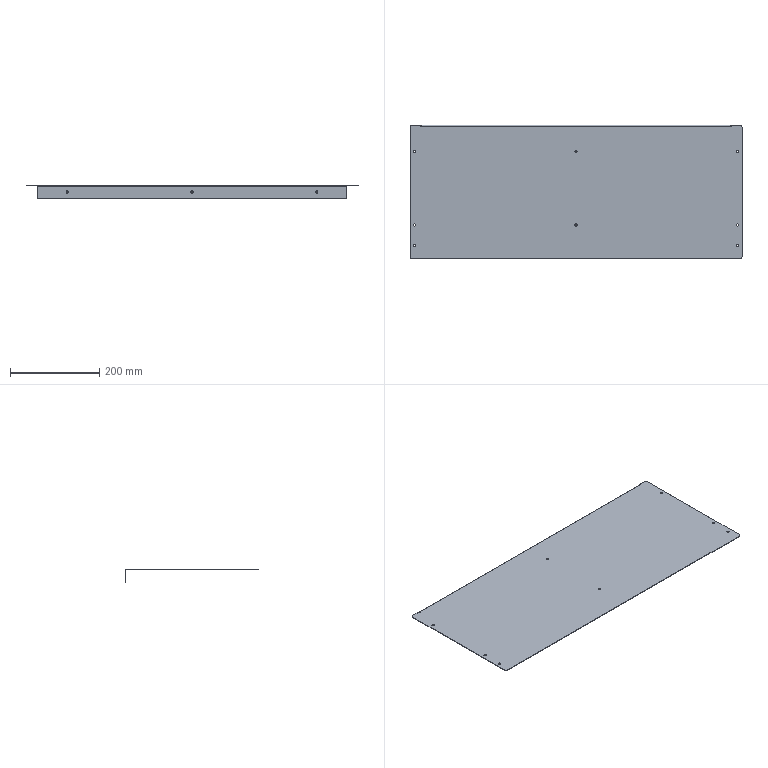Part | SolidWorks | features EdgeFlange 2, HoleWzd 2, Fillet 1, FlatPattern 1, SMBaseFlange 1, SheetMetal 1 | 1 solid | 50 faces | box 745 x 300 x 30 mm | volume 291345 mm3 | cylinder 30 | plane 20 | commonest cylinder face diameters 5 x22 10 x6 2 x1 4.4 x1